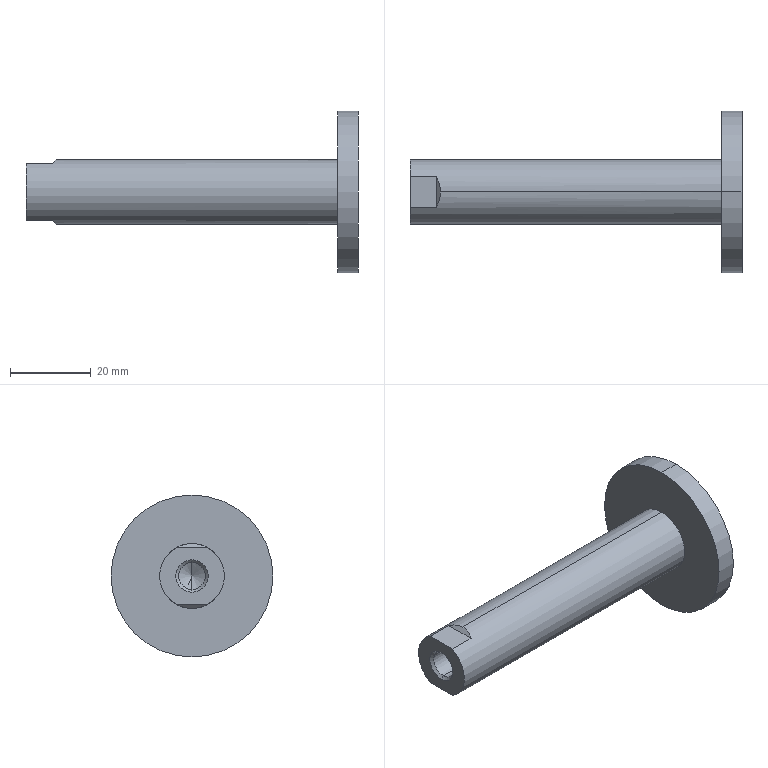Part | STEP file | _CDQ2F40-50-D-A93(0_0)_CYROD.stp | 1 solid | 17 faces | box 82 x 40 x 40 mm | volume 21214 mm3 | plane 7 | cylinder 6 | cone 4 | commonest cylinder face diameters 6.647 x2 16 x2 40 x2
STEP:
#1=CARTESIAN_POINT('',(0.,0.,0.));
#2=DIRECTION('',(0.,0.,1.));
#3=DIRECTION('',(1.,0.,0.));
#4=AXIS2_PLACEMENT_3D('',#1,#2,#3);
#5=CARTESIAN_POINT('',(-4.,0.,3.323));
#6=VERTEX_POINT('',#5);
#7=CARTESIAN_POINT('',(-4.,0.,-3.324));
#8=VERTEX_POINT('',#7);
#9=CARTESIAN_POINT('',(-4.,0.,0.));
#10=DIRECTION('',(1.,0.,0.));
#11=DIRECTION('',(0.,0.,-1.));
#12=AXIS2_PLACEMENT_3D('',#9,#10,#11);
#13=CIRCLE('',#12,3.324);
#14=CARTESIAN_POINT('',(-3.081,0.,0.));
#15=DIRECTION('',(-1.,0.,0.));
#16=DIRECTION('',(0.,0.,1.));
#17=AXIS2_PLACEMENT_3D('',#14,#15,#16);
#18=CONICAL_SURFACE('',#17,1.732,1.047);
#19=CARTESIAN_POINT('',(9.425,0.9188));
#20=DIRECTION('',(-1.,0.));
#21=VECTOR('',#20,1.);
#22=LINE('',#19,#21);
#23=(GEOMETRIC_REPRESENTATION_CONTEXT(2)PARAMETRIC_REPRESENTATION_CONTEXT()REPRESENTATION_CONTEXT('',''));
#24=DEFINITIONAL_REPRESENTATION('',(#22),#23);
#25=PCURVE('',#18,#24);
#26=CARTESIAN_POINT('',(65.,0.,0.));
#27=DIRECTION('',(-1.,0.,0.));
#28=DIRECTION('',(0.,0.,-1.));
#29=AXIS2_PLACEMENT_3D('',#26,#27,#28);
#30=CYLINDRICAL_SURFACE('',#29,3.324);
#31=CARTESIAN_POINT('',(6.283,69.));
#32=DIRECTION('',(-1.,0.));
#33=VECTOR('',#32,1.);
#34=LINE('',#31,#33);
#35=(GEOMETRIC_REPRESENTATION_CONTEXT(2)PARAMETRIC_REPRESENTATION_CONTEXT()REPRESENTATION_CONTEXT('',''));
#36=DEFINITIONAL_REPRESENTATION('',(#34),#35);
#37=PCURVE('',#30,#36);
#38=SURFACE_CURVE('',#13,(#25,#37),.PCURVE_S1.);
#39=EDGE_CURVE('',#6,#8,#38,.T.);
#40=ORIENTED_EDGE('',*,*,#39,.T.);
#41=CARTESIAN_POINT('',(-2.081,0.,0.));
#42=VERTEX_POINT('',#41);
#43=CARTESIAN_POINT('',(-3.081,0.,-1.732));
#44=DIRECTION('',(-0.5,0.,-0.866));
#45=VECTOR('',#44,1.);
#46=LINE('',#43,#45);
#47=CARTESIAN_POINT('',(3.142,0.));
#48=DIRECTION('',(0.,1.));
#49=VECTOR('',#48,1.);
#50=LINE('',#47,#49);
#51=(GEOMETRIC_REPRESENTATION_CONTEXT(2)PARAMETRIC_REPRESENTATION_CONTEXT()REPRESENTATION_CONTEXT('',''));
#52=DEFINITIONAL_REPRESENTATION('',(#50),#51);
#53=PCURVE('',#18,#52);
#54=CARTESIAN_POINT('',(-3.081,0.,0.));
#55=DIRECTION('',(-1.,0.,0.));
#56=DIRECTION('',(0.,0.,1.));
#57=AXIS2_PLACEMENT_3D('',#54,#55,#56);
#58=CONICAL_SURFACE('',#57,1.732,1.047);
#59=CARTESIAN_POINT('',(3.142,0.));
#60=DIRECTION('',(0.,1.));
#61=VECTOR('',#60,1.);
#62=LINE('',#59,#61);
#63=(GEOMETRIC_REPRESENTATION_CONTEXT(2)PARAMETRIC_REPRESENTATION_CONTEXT()REPRESENTATION_CONTEXT('',''));
#64=DEFINITIONAL_REPRESENTATION('',(#62),#63);
#65=PCURVE('',#58,#64);
#66=SURFACE_CURVE('',#46,(#53,#65),.PCURVE_S1.);
#67=EDGE_CURVE('',#42,#8,#66,.T.);
#68=ORIENTED_EDGE('',*,*,#67,.F.);
#69=CARTESIAN_POINT('',(-3.081,0.,1.732));
#70=DIRECTION('',(-0.5,0.,0.866));
#71=VECTOR('',#70,1.);
#72=LINE('',#69,#71);
#73=CARTESIAN_POINT('',(6.283,0.));
#74=DIRECTION('',(0.,1.));
#75=VECTOR('',#74,1.);
#76=LINE('',#73,#75);
#77=(GEOMETRIC_REPRESENTATION_CONTEXT(2)PARAMETRIC_REPRESENTATION_CONTEXT()REPRESENTATION_CONTEXT('',''));
#78=DEFINITIONAL_REPRESENTATION('',(#76),#77);
#79=PCURVE('',#18,#78);
#80=CARTESIAN_POINT('',(0.,0.));
#81=DIRECTION('',(0.,1.));
#82=VECTOR('',#81,1.);
#83=LINE('',#80,#82);
#84=(GEOMETRIC_REPRESENTATION_CONTEXT(2)PARAMETRIC_REPRESENTATION_CONTEXT()REPRESENTATION_CONTEXT('',''));
#85=DEFINITIONAL_REPRESENTATION('',(#83),#84);
#86=PCURVE('',#58,#85);
#87=SURFACE_CURVE('',#72,(#79,#86),.PCURVE_S1.);
#88=EDGE_CURVE('',#42,#6,#87,.T.);
#89=ORIENTED_EDGE('',*,*,#88,.T.);
#90=EDGE_LOOP('',(#40,#68,#89));
#91=FACE_BOUND('',#90,.F.);
#92=ADVANCED_FACE('',(#91),#18,.F.);
#93=CARTESIAN_POINT('',(-10.5,3.873,-7.));
#94=VERTEX_POINT('',#93);
#95=CARTESIAN_POINT('',(-9.5,0.,-8.));
#96=VERTEX_POINT('',#95);
#97=CARTESIAN_POINT('',(-10.5,3.873,-7.));
#98=CARTESIAN_POINT('',(-9.841,2.681,-7.659));
#99=CARTESIAN_POINT('',(-9.5,1.362,-8.));
#100=CARTESIAN_POINT('',(-9.5,0.,-8.));
#101=(BOUNDED_CURVE()B_SPLINE_CURVE(3,(#97,#98,#99,#100),.UNSPECIFIED.,.F.,.F.)B_SPLINE_CURVE_WITH_KNOTS((4,4),(5.778,6.283),.PIECEWISE_BEZIER_KNOTS.)CURVE()GEOMETRIC_REPRESENTATION_ITEM()RATIONAL_B_SPLINE_CURVE((1.,0.9788,0.9788,1.))REPRESENTATION_ITEM(''));
#102=CARTESIAN_POINT('',(-9.463,-4.26,-8.037));
#103=DIRECTION('',(-0.7071,0.,-0.7071));
#104=DIRECTION('',(-0.7071,0.,0.7071));
#105=AXIS2_PLACEMENT_3D('',#102,#103,#104);
#106=PLANE('',#105);
#107=CARTESIAN_POINT('',(1.466,8.133));
#108=CARTESIAN_POINT('',(0.5336,6.941));
#109=CARTESIAN_POINT('',(0.05199,5.622));
#110=CARTESIAN_POINT('',(0.05199,4.26));
#111=(BOUNDED_CURVE()B_SPLINE_CURVE(3,(#107,#108,#109,#110),.UNSPECIFIED.,.F.,.F.)B_SPLINE_CURVE_WITH_KNOTS((4,4),(5.778,6.283),.PIECEWISE_BEZIER_KNOTS.)CURVE()GEOMETRIC_REPRESENTATION_ITEM()RATIONAL_B_SPLINE_CURVE((1.,0.9788,0.9788,1.))REPRESENTATION_ITEM(''));
#112=(GEOMETRIC_REPRESENTATION_CONTEXT(2)PARAMETRIC_REPRESENTATION_CONTEXT()REPRESENTATION_CONTEXT('',''));
#113=DEFINITIONAL_REPRESENTATION('',(#111),#112);
#114=PCURVE('',#106,#113);
#115=CARTESIAN_POINT('',(65.,0.,0.));
#116=DIRECTION('',(-1.,0.,0.));
#117=DIRECTION('',(0.,0.,-1.));
#118=AXIS2_PLACEMENT_3D('',#115,#116,#117);
#119=CYLINDRICAL_SURFACE('',#118,8.);
#120=CARTESIAN_POINT('',(5.778,75.5));
#121=CARTESIAN_POINT('',(5.785,75.471));
#122=CARTESIAN_POINT('',(5.801,75.413));
#123=CARTESIAN_POINT('',(5.823,75.33));
#124=CARTESIAN_POINT('',(5.846,75.251));
#125=CARTESIAN_POINT('',(5.869,75.175));
#126=CARTESIAN_POINT('',(5.892,75.103));
#127=CARTESIAN_POINT('',(5.915,75.035));
#128=CARTESIAN_POINT('',(5.938,74.971));
#129=CARTESIAN_POINT('',(5.961,74.91));
#130=CARTESIAN_POINT('',(5.984,74.854));
#131=CARTESIAN_POINT('',(6.007,74.802));
#132=CARTESIAN_POINT('',(6.031,74.753));
#133=CARTESIAN_POINT('',(6.054,74.709));
#134=CARTESIAN_POINT('',(6.077,74.669));
#135=CARTESIAN_POINT('',(6.1,74.634));
#136=CARTESIAN_POINT('',(6.123,74.602));
#137=CARTESIAN_POINT('',(6.146,74.575));
#138=CARTESIAN_POINT('',(6.169,74.552));
#139=CARTESIAN_POINT('',(6.192,74.533));
#140=CARTESIAN_POINT('',(6.215,74.518));
#141=CARTESIAN_POINT('',(6.238,74.508));
#142=CARTESIAN_POINT('',(6.26,74.501));
#143=CARTESIAN_POINT('',(6.276,74.5));
#144=CARTESIAN_POINT('',(6.283,74.5));
#145=B_SPLINE_CURVE_WITH_KNOTS('',3,(#120,#121,#122,#123,#124,#125,#126,#127,#128,#129,#130,#131,#132,#133,#134,#135,#136,#137,#138,#139,#140,#141,#142,#143,#144),.UNSPECIFIED.,.F.,.F.,(4,1,1,1,1,1,1,1,1,1,1,1,1,1,1,1,1,1,1,1,1,1,4),(5.778,5.801,5.824,5.847,5.87,5.893,5.916,5.939,5.962,5.985,6.008,6.031,6.053,6.076,6.099,6.122,6.145,6.168,6.191,6.214,6.237,6.26,6.283),.QUASI_UNIFORM_KNOTS.);
#146=(GEOMETRIC_REPRESENTATION_CONTEXT(2)PARAMETRIC_REPRESENTATION_CONTEXT()REPRESENTATION_CONTEXT('',''));
#147=DEFINITIONAL_REPRESENTATION('',(#145),#146);
#148=PCURVE('',#119,#147);
#149=SURFACE_CURVE('',#101,(#114,#148),.PCURVE_S1.);
#150=EDGE_CURVE('',#94,#96,#149,.T.);
#151=ORIENTED_EDGE('',*,*,#150,.T.);
#152=CARTESIAN_POINT('',(-10.5,-3.873,-7.));
#153=VERTEX_POINT('',#152);
#154=CARTESIAN_POINT('',(-9.5,0.,-8.));
#155=CARTESIAN_POINT('',(-9.5,-1.362,-8.));
#156=CARTESIAN_POINT('',(-9.841,-2.681,-7.659));
#157=CARTESIAN_POINT('',(-10.5,-3.873,-7.));
#158=(BOUNDED_CURVE()B_SPLINE_CURVE(3,(#154,#155,#156,#157),.UNSPECIFIED.,.F.,.F.)B_SPLINE_CURVE_WITH_KNOTS((4,4),(0.,0.5054),.PIECEWISE_BEZIER_KNOTS.)CURVE()GEOMETRIC_REPRESENTATION_ITEM()RATIONAL_B_SPLINE_CURVE((1.,0.9788,0.9788,1.))REPRESENTATION_ITEM(''));
#159=CARTESIAN_POINT('',(0.05199,4.26));
#160=CARTESIAN_POINT('',(0.05199,2.898));
#161=CARTESIAN_POINT('',(0.5336,1.579));
#162=CARTESIAN_POINT('',(1.466,0.3873));
#163=(BOUNDED_CURVE()B_SPLINE_CURVE(3,(#159,#160,#161,#162),.UNSPECIFIED.,.F.,.F.)B_SPLINE_CURVE_WITH_KNOTS((4,4),(0.,0.5054),.PIECEWISE_BEZIER_KNOTS.)CURVE()GEOMETRIC_REPRESENTATION_ITEM()RATIONAL_B_SPLINE_CURVE((1.,0.9788,0.9788,1.))REPRESENTATION_ITEM(''));
#164=(GEOMETRIC_REPRESENTATION_CONTEXT(2)PARAMETRIC_REPRESENTATION_CONTEXT()REPRESENTATION_CONTEXT('',''));
#165=DEFINITIONAL_REPRESENTATION('',(#163),#164);
#166=PCURVE('',#106,#165);
#167=CARTESIAN_POINT('',(65.,0.,0.));
#168=DIRECTION('',(-1.,0.,0.));
#169=DIRECTION('',(0.,0.,-1.));
#170=AXIS2_PLACEMENT_3D('',#167,#168,#169);
#171=CYLINDRICAL_SURFACE('',#170,8.);
#172=CARTESIAN_POINT('',(0.,74.5));
#173=CARTESIAN_POINT('',(0.007576,74.5));
#174=CARTESIAN_POINT('',(0.02275,74.501));
#175=CARTESIAN_POINT('',(0.04557,74.508));
#176=CARTESIAN_POINT('',(0.06844,74.518));
#177=CARTESIAN_POINT('',(0.09137,74.533));
#178=CARTESIAN_POINT('',(0.1143,74.552));
#179=CARTESIAN_POINT('',(0.1373,74.575));
#180=CARTESIAN_POINT('',(0.1604,74.602));
#181=CARTESIAN_POINT('',(0.1834,74.634));
#182=CARTESIAN_POINT('',(0.2065,74.669));
#183=CARTESIAN_POINT('',(0.2296,74.709));
#184=CARTESIAN_POINT('',(0.2527,74.753));
#185=CARTESIAN_POINT('',(0.2758,74.802));
#186=CARTESIAN_POINT('',(0.2989,74.854));
#187=CARTESIAN_POINT('',(0.3219,74.91));
#188=CARTESIAN_POINT('',(0.345,74.971));
#189=CARTESIAN_POINT('',(0.368,75.035));
#190=CARTESIAN_POINT('',(0.391,75.103));
#191=CARTESIAN_POINT('',(0.414,75.175));
#192=CARTESIAN_POINT('',(0.4369,75.251));
#193=CARTESIAN_POINT('',(0.4598,75.33));
#194=CARTESIAN_POINT('',(0.4826,75.413));
#195=CARTESIAN_POINT('',(0.4978,75.471));
#196=CARTESIAN_POINT('',(0.5054,75.5));
#197=B_SPLINE_CURVE_WITH_KNOTS('',3,(#172,#173,#174,#175,#176,#177,#178,#179,#180,#181,#182,#183,#184,#185,#186,#187,#188,#189,#190,#191,#192,#193,#194,#195,#196),.UNSPECIFIED.,.F.,.F.,(4,1,1,1,1,1,1,1,1,1,1,1,1,1,1,1,1,1,1,1,1,1,4),(0.,0.02297,0.04594,0.06891,0.09188,0.1149,0.1378,0.1608,0.1838,0.2067,0.2297,0.2527,0.2757,0.2986,0.3216,0.3446,0.3675,0.3905,0.4135,0.4364,0.4594,0.4824,0.5054),.QUASI_UNIFORM_KNOTS.);
#198=(GEOMETRIC_REPRESENTATION_CONTEXT(2)PARAMETRIC_REPRESENTATION_CONTEXT()REPRESENTATION_CONTEXT('',''));
#199=DEFINITIONAL_REPRESENTATION('',(#197),#198);
#200=PCURVE('',#171,#199);
#201=SURFACE_CURVE('',#158,(#166,#200),.PCURVE_S1.);
#202=EDGE_CURVE('',#96,#153,#201,.T.);
#203=ORIENTED_EDGE('',*,*,#202,.T.);
#204=CARTESIAN_POINT('',(-10.5,3.873,-7.));
#205=DIRECTION('',(0.,-1.,0.));
#206=VECTOR('',#205,1.);
#207=LINE('',#204,#206);
#208=CARTESIAN_POINT('',(1.466,8.133));
#209=DIRECTION('',(0.,-1.));
#210=VECTOR('',#209,1.);
#211=LINE('',#208,#210);
#212=(GEOMETRIC_REPRESENTATION_CONTEXT(2)PARAMETRIC_REPRESENTATION_CONTEXT()REPRESENTATION_CONTEXT('',''));
#213=DEFINITIONAL_REPRESENTATION('',(#211),#212);
#214=PCURVE('',#106,#213);
#215=CARTESIAN_POINT('',(-10.175,-4.26,-7.));
#216=DIRECTION('',(0.,0.,-1.));
#217=DIRECTION('',(0.,-1.,0.));
#218=AXIS2_PLACEMENT_3D('',#215,#216,#217);
#219=PLANE('',#218);
#220=CARTESIAN_POINT('',(-8.133,0.325));
#221=DIRECTION('',(1.,0.));
#222=VECTOR('',#221,1.);
#223=LINE('',#220,#222);
#224=(GEOMETRIC_REPRESENTATION_CONTEXT(2)PARAMETRIC_REPRESENTATION_CONTEXT()REPRESENTATION_CONTEXT('',''));
#225=DEFINITIONAL_REPRESENTATION('',(#223),#224);
#226=PCURVE('',#219,#225);
#227=SURFACE_CURVE('',#207,(#214,#226),.PCURVE_S1.);
#228=EDGE_CURVE('',#94,#153,#227,.T.);
#229=ORIENTED_EDGE('',*,*,#228,.F.);
#230=EDGE_LOOP('',(#151,#203,#229));
#231=FACE_BOUND('',#230,.T.);
#232=ADVANCED_FACE('',(#231),#106,.T.);
#233=CARTESIAN_POINT('',(-17.,3.873,-7.));
#234=VERTEX_POINT('',#233);
#235=CARTESIAN_POINT('',(-17.,3.873,-7.));
#236=DIRECTION('',(1.,0.,0.));
#237=VECTOR('',#236,1.);
#238=LINE('',#235,#237);
#239=CARTESIAN_POINT('',(-8.133,6.825));
#240=DIRECTION('',(0.,-1.));
#241=VECTOR('',#240,1.);
#242=LINE('',#239,#241);
#243=(GEOMETRIC_REPRESENTATION_CONTEXT(2)PARAMETRIC_REPRESENTATION_CONTEXT()REPRESENTATION_CONTEXT('',''));
#244=DEFINITIONAL_REPRESENTATION('',(#242),#243);
#245=PCURVE('',#219,#244);
#246=CARTESIAN_POINT('',(5.778,82.));
#247=DIRECTION('',(0.,-1.));
#248=VECTOR('',#247,1.);
#249=LINE('',#246,#248);
#250=(GEOMETRIC_REPRESENTATION_CONTEXT(2)PARAMETRIC_REPRESENTATION_CONTEXT()REPRESENTATION_CONTEXT('',''));
#251=DEFINITIONAL_REPRESENTATION('',(#249),#250);
#252=PCURVE('',#119,#251);
#253=SURFACE_CURVE('',#238,(#245,#252),.PCURVE_S1.);
#254=EDGE_CURVE('',#234,#94,#253,.T.);
#255=ORIENTED_EDGE('',*,*,#254,.T.);
#256=ORIENTED_EDGE('',*,*,#228,.T.);
#257=CARTESIAN_POINT('',(-17.,-3.873,-7.));
#258=VERTEX_POINT('',#257);
#259=CARTESIAN_POINT('',(-17.,-3.873,-7.));
#260=DIRECTION('',(-1.,0.,0.));
#261=VECTOR('',#260,1.);
#262=LINE('',#259,#261);
#263=CARTESIAN_POINT('',(-0.3873,6.825));
#264=DIRECTION('',(0.,1.));
#265=VECTOR('',#264,1.);
#266=LINE('',#263,#265);
#267=(GEOMETRIC_REPRESENTATION_CONTEXT(2)PARAMETRIC_REPRESENTATION_CONTEXT()REPRESENTATION_CONTEXT('',''));
#268=DEFINITIONAL_REPRESENTATION('',(#266),#267);
#269=PCURVE('',#219,#268);
#270=CARTESIAN_POINT('',(0.5054,82.));
#271=DIRECTION('',(0.,1.));
#272=VECTOR('',#271,1.);
#273=LINE('',#270,#272);
#274=(GEOMETRIC_REPRESENTATION_CONTEXT(2)PARAMETRIC_REPRESENTATION_CONTEXT()REPRESENTATION_CONTEXT('',''));
#275=DEFINITIONAL_REPRESENTATION('',(#273),#274);
#276=PCURVE('',#171,#275);
#277=SURFACE_CURVE('',#262,(#269,#276),.PCURVE_S1.);
#278=EDGE_CURVE('',#153,#258,#277,.T.);
#279=ORIENTED_EDGE('',*,*,#278,.T.);
#280=CARTESIAN_POINT('',(-17.,3.873,-7.));
#281=DIRECTION('',(0.,-1.,0.));
#282=VECTOR('',#281,1.);
#283=LINE('',#280,#282);
#284=CARTESIAN_POINT('',(-8.133,6.825));
#285=DIRECTION('',(1.,0.));
#286=VECTOR('',#285,1.);
#287=LINE('',#284,#286);
#288=(GEOMETRIC_REPRESENTATION_CONTEXT(2)PARAMETRIC_REPRESENTATION_CONTEXT()REPRESENTATION_CONTEXT('',''));
#289=DEFINITIONAL_REPRESENTATION('',(#287),#288);
#290=PCURVE('',#219,#289);
#291=CARTESIAN_POINT('',(-17.,-8.8,7.7));
#292=DIRECTION('',(1.,0.,0.));
#293=DIRECTION('',(0.,1.,0.));
#294=AXIS2_PLACEMENT_3D('',#291,#292,#293);
#295=PLANE('',#294);
#296=CARTESIAN_POINT('',(12.673,-14.7));
#297=DIRECTION('',(-1.,0.));
#298=VECTOR('',#297,1.);
#299=LINE('',#296,#298);
#300=(GEOMETRIC_REPRESENTATION_CONTEXT(2)PARAMETRIC_REPRESENTATION_CONTEXT()REPRESENTATION_CONTEXT('',''));
#301=DEFINITIONAL_REPRESENTATION('',(#299),#300);
#302=PCURVE('',#295,#301);
#303=SURFACE_CURVE('',#283,(#290,#302),.PCURVE_S1.);
#304=EDGE_CURVE('',#234,#258,#303,.T.);
#305=ORIENTED_EDGE('',*,*,#304,.F.);
#306=EDGE_LOOP('',(#255,#256,#279,#305));
#307=FACE_BOUND('',#306,.T.);
#308=ADVANCED_FACE('',(#307),#219,.T.);
#309=CARTESIAN_POINT('',(-17.,-3.873,7.));
#310=VERTEX_POINT('',#309);
#311=CARTESIAN_POINT('',(-10.5,-3.873,7.));
#312=VERTEX_POINT('',#311);
#313=CARTESIAN_POINT('',(-17.,-3.873,7.));
#314=DIRECTION('',(1.,0.,0.));
#315=VECTOR('',#314,1.);
#316=LINE('',#313,#315);
#317=CARTESIAN_POINT('',(-17.325,-4.26,7.));
#318=DIRECTION('',(0.,0.,1.));
#319=DIRECTION('',(1.,0.,0.));
#320=AXIS2_PLACEMENT_3D('',#317,#318,#319);
#321=PLANE('',#320);
#322=CARTESIAN_POINT('',(0.325,0.3873));
#323=DIRECTION('',(1.,0.));
#324=VECTOR('',#323,1.);
#325=LINE('',#322,#324);
#326=(GEOMETRIC_REPRESENTATION_CONTEXT(2)PARAMETRIC_REPRESENTATION_CONTEXT()REPRESENTATION_CONTEXT('',''));
#327=DEFINITIONAL_REPRESENTATION('',(#325),#326);
#328=PCURVE('',#321,#327);
#329=CARTESIAN_POINT('',(2.636,82.));
#330=DIRECTION('',(0.,-1.));
#331=VECTOR('',#330,1.);
#332=LINE('',#329,#331);
#333=(GEOMETRIC_REPRESENTATION_CONTEXT(2)PARAMETRIC_REPRESENTATION_CONTEXT()REPRESENTATION_CONTEXT('',''));
#334=DEFINITIONAL_REPRESENTATION('',(#332),#333);
#335=PCURVE('',#171,#334);
#336=SURFACE_CURVE('',#316,(#328,#335),.PCURVE_S1.);
#337=EDGE_CURVE('',#310,#312,#336,.T.);
#338=ORIENTED_EDGE('',*,*,#337,.T.);
#339=CARTESIAN_POINT('',(-10.5,3.873,7.));
#340=VERTEX_POINT('',#339);
#341=CARTESIAN_POINT('',(-10.5,3.873,7.));
#342=DIRECTION('',(0.,-1.,0.));
#343=VECTOR('',#342,1.);
#344=LINE('',#341,#343);
#345=CARTESIAN_POINT('',(6.825,8.133));
#346=DIRECTION('',(0.,-1.));
#347=VECTOR('',#346,1.);
#348=LINE('',#345,#347);
#349=(GEOMETRIC_REPRESENTATION_CONTEXT(2)PARAMETRIC_REPRESENTATION_CONTEXT()REPRESENTATION_CONTEXT('',''));
#350=DEFINITIONAL_REPRESENTATION('',(#348),#349);
#351=PCURVE('',#321,#350);
#352=CARTESIAN_POINT('',(-10.549,-4.26,6.951));
#353=DIRECTION('',(-0.7071,0.,0.7071));
#354=DIRECTION('',(0.,1.,0.));
#355=AXIS2_PLACEMENT_3D('',#352,#353,#354);
#356=PLANE('',#355);
#357=CARTESIAN_POINT('',(8.133,-0.06982));
#358=DIRECTION('',(-1.,0.));
#359=VECTOR('',#358,1.);
#360=LINE('',#357,#359);
#361=(GEOMETRIC_REPRESENTATION_CONTEXT(2)PARAMETRIC_REPRESENTATION_CONTEXT()REPRESENTATION_CONTEXT('',''));
#362=DEFINITIONAL_REPRESENTATION('',(#360),#361);
#363=PCURVE('',#356,#362);
#364=SURFACE_CURVE('',#344,(#351,#363),.PCURVE_S1.);
#365=EDGE_CURVE('',#340,#312,#364,.T.);
#366=ORIENTED_EDGE('',*,*,#365,.F.);
#367=CARTESIAN_POINT('',(-17.,3.873,7.));
#368=VERTEX_POINT('',#367);
#369=CARTESIAN_POINT('',(-17.,3.873,7.));
#370=DIRECTION('',(-1.,0.,0.));
#371=VECTOR('',#370,1.);
#372=LINE('',#369,#371);
#373=CARTESIAN_POINT('',(0.325,8.133));
#374=DIRECTION('',(-1.,0.));
#375=VECTOR('',#374,1.);
#376=LINE('',#373,#375);
#377=(GEOMETRIC_REPRESENTATION_CONTEXT(2)PARAMETRIC_REPRESENTATION_CONTEXT()REPRESENTATION_CONTEXT('',''));
#378=DEFINITIONAL_REPRESENTATION('',(#376),#377);
#379=PCURVE('',#321,#378);
#380=CARTESIAN_POINT('',(3.647,82.));
#381=DIRECTION('',(0.,1.));
#382=VECTOR('',#381,1.);
#383=LINE('',#380,#382);
#384=(GEOMETRIC_REPRESENTATION_CONTEXT(2)PARAMETRIC_REPRESENTATION_CONTEXT()REPRESENTATION_CONTEXT('',''));
#385=DEFINITIONAL_REPRESENTATION('',(#383),#384);
#386=PCURVE('',#119,#385);
#387=SURFACE_CURVE('',#372,(#379,#386),.PCURVE_S1.);
#388=EDGE_CURVE('',#340,#368,#387,.T.);
#389=ORIENTED_EDGE('',*,*,#388,.T.);
#390=CARTESIAN_POINT('',(-17.,3.873,7.));
#391=DIRECTION('',(0.,-1.,0.));
#392=VECTOR('',#391,1.);
#393=LINE('',#390,#392);
#394=CARTESIAN_POINT('',(0.325,8.133));
#395=DIRECTION('',(0.,-1.));
#396=VECTOR('',#395,1.);
#397=LINE('',#394,#396);
#398=(GEOMETRIC_REPRESENTATION_CONTEXT(2)PARAMETRIC_REPRESENTATION_CONTEXT()REPRESENTATION_CONTEXT('',''));
#399=DEFINITIONAL_REPRESENTATION('',(#397),#398);
#400=PCURVE('',#321,#399);
#401=CARTESIAN_POINT('',(12.673,-0.7));
#402=DIRECTION('',(-1.,0.));
#403=VECTOR('',#402,1.);
#404=LINE('',#401,#403);
#405=(GEOMETRIC_REPRESENTATION_CONTEXT(2)PARAMETRIC_REPRESENTATION_CONTEXT()REPRESENTATION_CONTEXT('',''));
#406=DEFINITIONAL_REPRESENTATION('',(#404),#405);
#407=PCURVE('',#295,#406);
#408=SURFACE_CURVE('',#393,(#400,#407),.PCURVE_S1.);
#409=EDGE_CURVE('',#368,#310,#408,.T.);
#410=ORIENTED_EDGE('',*,*,#409,.T.);
#411=EDGE_LOOP('',(#338,#366,#389,#410));
#412=FACE_BOUND('',#411,.T.);
#413=ADVANCED_FACE('',(#412),#321,.T.);
#414=CARTESIAN_POINT('',(-9.5,0.,8.));
#415=VERTEX_POINT('',#414);
#416=CARTESIAN_POINT('',(-10.5,-3.873,7.));
#417=CARTESIAN_POINT('',(-9.841,-2.681,7.659));
#418=CARTESIAN_POINT('',(-9.5,-1.362,8.));
#419=CARTESIAN_POINT('',(-9.5,0.,8.));
#420=(BOUNDED_CURVE()B_SPLINE_CURVE(3,(#416,#417,#418,#419),.UNSPECIFIED.,.F.,.F.)B_SPLINE_CURVE_WITH_KNOTS((4,4),(5.778,6.283),.PIECEWISE_BEZIER_KNOTS.)CURVE()GEOMETRIC_REPRESENTATION_ITEM()RATIONAL_B_SPLINE_CURVE((1.,0.9788,0.9788,1.))REPRESENTATION_ITEM(''));
#421=CARTESIAN_POINT('',(0.3873,-0.06982));
#422=CARTESIAN_POINT('',(1.579,-1.002));
#423=CARTESIAN_POINT('',(2.898,-1.484));
#424=CARTESIAN_POINT('',(4.26,-1.484));
#425=(BOUNDED_CURVE()B_SPLINE_CURVE(3,(#421,#422,#423,#424),.UNSPECIFIED.,.F.,.F.)B_SPLINE_CURVE_WITH_KNOTS((4,4),(5.778,6.283),.PIECEWISE_BEZIER_KNOTS.)CURVE()GEOMETRIC_REPRESENTATION_ITEM()RATIONAL_B_SPLINE_CURVE((1.,0.9788,0.9788,1.))REPRESENTATION_ITEM(''));
#426=(GEOMETRIC_REPRESENTATION_CONTEXT(2)PARAMETRIC_REPRESENTATION_CONTEXT()REPRESENTATION_CONTEXT('',''));
#427=DEFINITIONAL_REPRESENTATION('',(#425),#426);
#428=PCURVE('',#356,#427);
#429=CARTESIAN_POINT('',(2.636,75.5));
#430=CARTESIAN_POINT('',(2.644,75.471));
#431=CARTESIAN_POINT('',(2.659,75.413));
#432=CARTESIAN_POINT('',(2.682,75.33));
#433=CARTESIAN_POINT('',(2.705,75.251));
#434=CARTESIAN_POINT('',(2.728,75.175));
#435=CARTESIAN_POINT('',(2.751,75.103));
#436=CARTESIAN_POINT('',(2.774,75.035));
#437=CARTESIAN_POINT('',(2.797,74.971));
#438=CARTESIAN_POINT('',(2.82,74.91));
#439=CARTESIAN_POINT('',(2.843,74.854));
#440=CARTESIAN_POINT('',(2.866,74.802));
#441=CARTESIAN_POINT('',(2.889,74.753));
#442=CARTESIAN_POINT('',(2.912,74.709));
#443=CARTESIAN_POINT('',(2.935,74.669));
#444=CARTESIAN_POINT('',(2.958,74.634));
#445=CARTESIAN_POINT('',(2.981,74.602));
#446=CARTESIAN_POINT('',(3.004,74.575));
#447=CARTESIAN_POINT('',(3.027,74.552));
#448=CARTESIAN_POINT('',(3.05,74.533));
#449=CARTESIAN_POINT('',(3.073,74.518));
#450=CARTESIAN_POINT('',(3.096,74.508));
#451=CARTESIAN_POINT('',(3.119,74.501));
#452=CARTESIAN_POINT('',(3.134,74.5));
#453=CARTESIAN_POINT('',(3.142,74.5));
#454=B_SPLINE_CURVE_WITH_KNOTS('',3,(#429,#430,#431,#432,#433,#434,#435,#436,#437,#438,#439,#440,#441,#442,#443,#444,#445,#446,#447,#448,#449,#450,#451,#452,#453),.UNSPECIFIED.,.F.,.F.,(4,1,1,1,1,1,1,1,1,1,1,1,1,1,1,1,1,1,1,1,1,1,4),(5.778,5.801,5.824,5.847,5.87,5.893,5.916,5.939,5.962,5.985,6.008,6.031,6.053,6.076,6.099,6.122,6.145,6.168,6.191,6.214,6.237,6.26,6.283),.QUASI_UNIFORM_KNOTS.);
#455=(GEOMETRIC_REPRESENTATION_CONTEXT(2)PARAMETRIC_REPRESENTATION_CONTEXT()REPRESENTATION_CONTEXT('',''));
#456=DEFINITIONAL_REPRESENTATION('',(#454),#455);
#457=PCURVE('',#171,#456);
#458=SURFACE_CURVE('',#420,(#428,#457),.PCURVE_S1.);
#459=EDGE_CURVE('',#312,#415,#458,.T.);
#460=ORIENTED_EDGE('',*,*,#459,.T.);
#461=CARTESIAN_POINT('',(-9.5,0.,8.));
#462=CARTESIAN_POINT('',(-9.5,1.362,8.));
#463=CARTESIAN_POINT('',(-9.841,2.681,7.659));
#464=CARTESIAN_POINT('',(-10.5,3.873,7.));
#465=(BOUNDED_CURVE()B_SPLINE_CURVE(3,(#461,#462,#463,#464),.UNSPECIFIED.,.F.,.F.)B_SPLINE_CURVE_WITH_KNOTS((4,4),(0.,0.5054),.PIECEWISE_BEZIER_KNOTS.)CURVE()GEOMETRIC_REPRESENTATION_ITEM()RATIONAL_B_SPLINE_CURVE((1.,0.9788,0.9788,1.))REPRESENTATION_ITEM(''));
#466=CARTESIAN_POINT('',(4.26,-1.484));
#467=CARTESIAN_POINT('',(5.622,-1.484));
#468=CARTESIAN_POINT('',(6.941,-1.002));
#469=CARTESIAN_POINT('',(8.133,-0.06982));
#470=(BOUNDED_CURVE()B_SPLINE_CURVE(3,(#466,#467,#468,#469),.UNSPECIFIED.,.F.,.F.)B_SPLINE_CURVE_WITH_KNOTS((4,4),(0.,0.5054),.PIECEWISE_BEZIER_KNOTS.)CURVE()GEOMETRIC_REPRESENTATION_ITEM()RATIONAL_B_SPLINE_CURVE((1.,0.9788,0.9788,1.))REPRESENTATION_ITEM(''));
#471=(GEOMETRIC_REPRESENTATION_CONTEXT(2)PARAMETRIC_REPRESENTATION_CONTEXT()REPRESENTATION_CONTEXT('',''));
#472=DEFINITIONAL_REPRESENTATION('',(#470),#471);
#473=PCURVE('',#356,#472);
#474=CARTESIAN_POINT('',(3.142,74.5));
#475=CARTESIAN_POINT('',(3.149,74.5));
#476=CARTESIAN_POINT('',(3.164,74.501));
#477=CARTESIAN_POINT('',(3.187,74.508));
#478=CARTESIAN_POINT('',(3.21,74.518));
#479=CARTESIAN_POINT('',(3.233,74.533));
#480=CARTESIAN_POINT('',(3.256,74.552));
#481=CARTESIAN_POINT('',(3.279,74.575));
#482=CARTESIAN_POINT('',(3.302,74.602));
#483=CARTESIAN_POINT('',(3.325,74.634));
#484=CARTESIAN_POINT('',(3.348,74.669));
#485=CARTESIAN_POINT('',(3.371,74.709));
#486=CARTESIAN_POINT('',(3.394,74.753));
#487=CARTESIAN_POINT('',(3.417,74.802));
#488=CARTESIAN_POINT('',(3.44,74.854));
#489=CARTESIAN_POINT('',(3.464,74.91));
#490=CARTESIAN_POINT('',(3.487,74.971));
#491=CARTESIAN_POINT('',(3.51,75.035));
#492=CARTESIAN_POINT('',(3.533,75.103));
#493=CARTESIAN_POINT('',(3.556,75.175));
#494=CARTESIAN_POINT('',(3.579,75.251));
#495=CARTESIAN_POINT('',(3.601,75.33));
#496=CARTESIAN_POINT('',(3.624,75.413));
#497=CARTESIAN_POINT('',(3.639,75.471));
#498=CARTESIAN_POINT('',(3.647,75.5));
#499=B_SPLINE_CURVE_WITH_KNOTS('',3,(#474,#475,#476,#477,#478,#479,#480,#481,#482,#483,#484,#485,#486,#487,#488,#489,#490,#491,#492,#493,#494,#495,#496,#497,#498),.UNSPECIFIED.,.F.,.F.,(4,1,1,1,1,1,1,1,1,1,1,1,1,1,1,1,1,1,1,1,1,1,4),(0.,0.02297,0.04594,0.06891,0.09188,0.1149,0.1378,0.1608,0.1838,0.2067,0.2297,0.2527,0.2757,0.2986,0.3216,0.3446,0.3675,0.3905,0.4135,0.4364,0.4594,0.4824,0.5054),.QUASI_UNIFORM_KNOTS.);
#500=(GEOMETRIC_REPRESENTATION_CONTEXT(2)PARAMETRIC_REPRESENTATION_CONTEXT()REPRESENTATION_CONTEXT('',''));
#501=DEFINITIONAL_REPRESENTATION('',(#499),#500);
#502=PCURVE('',#119,#501);
#503=SURFACE_CURVE('',#465,(#473,#502),.PCURVE_S1.);
#504=EDGE_CURVE('',#415,#340,#503,.T.);
#505=ORIENTED_EDGE('',*,*,#504,.T.);
#506=ORIENTED_EDGE('',*,*,#365,.T.);
#507=EDGE_LOOP('',(#460,#505,#506));
#508=FACE_BOUND('',#507,.T.);
#509=ADVANCED_FACE('',(#508),#356,.T.);
#510=CARTESIAN_POINT('',(65.,0.,-20.));
#511=VERTEX_POINT('',#510);
#512=CARTESIAN_POINT('',(65.,0.,20.));
#513=VERTEX_POINT('',#512);
#514=CARTESIAN_POINT('',(65.,0.,0.));
#515=DIRECTION('',(1.,0.,0.));
#516=DIRECTION('',(0.,0.,-1.));
#517=AXIS2_PLACEMENT_3D('',#514,#515,#516);
#518=CIRCLE('',#517,20.);
#519=CARTESIAN_POINT('',(65.,-22.,-22.));
#520=DIRECTION('',(-1.,0.,0.));
#521=DIRECTION('',(0.,0.,1.));
#522=AXIS2_PLACEMENT_3D('',#519,#520,#521);
#523=PLANE('',#522);
#524=CARTESIAN_POINT('',(2.,22.));
#525=CARTESIAN_POINT('',(2.,56.641));
#526=CARTESIAN_POINT('',(32.,39.321));
#527=CARTESIAN_POINT('',(62.,22.));
#528=CARTESIAN_POINT('',(32.,4.679));
#529=CARTESIAN_POINT('',(2.,-12.641));
#530=CARTESIAN_POINT('',(2.,22.));
#531=(BOUNDED_CURVE()B_SPLINE_CURVE(2,(#524,#525,#526,#527,#528,#529,#530),.UNSPECIFIED.,.T.,.F.)B_SPLINE_CURVE_WITH_KNOTS((1,2,2,2,2,1),(-2.094,0.,2.094,4.189,6.283,8.378),.UNSPECIFIED.)CURVE()GEOMETRIC_REPRESENTATION_ITEM()RATIONAL_B_SPLINE_CURVE((1.,0.5,1.,0.5,1.,0.5,1.))REPRESENTATION_ITEM(''));
#532=(GEOMETRIC_REPRESENTATION_CONTEXT(2)PARAMETRIC_REPRESENTATION_CONTEXT()REPRESENTATION_CONTEXT('',''));
#533=DEFINITIONAL_REPRESENTATION('',(#531),#532);
#534=PCURVE('',#523,#533);
#535=CARTESIAN_POINT('',(65.25,0.,0.));
#536=DIRECTION('',(-1.,0.,0.));
#537=DIRECTION('',(0.,0.,-1.));
#538=AXIS2_PLACEMENT_3D('',#535,#536,#537);
#539=CYLINDRICAL_SURFACE('',#538,20.);
#540=CARTESIAN_POINT('',(6.283,0.25));
#541=DIRECTION('',(-1.,0.));
#542=VECTOR('',#541,1.);
#543=LINE('',#540,#542);
#544=(GEOMETRIC_REPRESENTATION_CONTEXT(2)PARAMETRIC_REPRESENTATION_CONTEXT()REPRESENTATION_CONTEXT('',''));
#545=DEFINITIONAL_REPRESENTATION('',(#543),#544);
#546=PCURVE('',#539,#545);
#547=SURFACE_CURVE('',#518,(#534,#546),.PCURVE_S1.);
#548=EDGE_CURVE('',#511,#513,#547,.T.);
#549=ORIENTED_EDGE('',*,*,#548,.T.);
#550=CARTESIAN_POINT('',(65.,0.,0.));
#551=DIRECTION('',(1.,0.,0.));
#552=DIRECTION('',(0.,0.,-1.));
#553=AXIS2_PLACEMENT_3D('',#550,#551,#552);
#554=CIRCLE('',#553,20.);
#555=CARTESIAN_POINT('',(2.,22.));
#556=CARTESIAN_POINT('',(2.,56.641));
#557=CARTESIAN_POINT('',(32.,39.321));
#558=CARTESIAN_POINT('',(62.,22.));
#559=CARTESIAN_POINT('',(32.,4.679));
#560=CARTESIAN_POINT('',(2.,-12.641));
#561=CARTESIAN_POINT('',(2.,22.));
#562=(BOUNDED_CURVE()B_SPLINE_CURVE(2,(#555,#556,#557,#558,#559,#560,#561),.UNSPECIFIED.,.T.,.F.)B_SPLINE_CURVE_WITH_KNOTS((1,2,2,2,2,1),(-2.094,0.,2.094,4.189,6.283,8.378),.UNSPECIFIED.)CURVE()GEOMETRIC_REPRESENTATION_ITEM()RATIONAL_B_SPLINE_CURVE((1.,0.5,1.,0.5,1.,0.5,1.))REPRESENTATION_ITEM(''));
#563=(GEOMETRIC_REPRESENTATION_CONTEXT(2)PARAMETRIC_REPRESENTATION_CONTEXT()REPRESENTATION_CONTEXT('',''));
#564=DEFINITIONAL_REPRESENTATION('',(#562),#563);
#565=PCURVE('',#523,#564);
#566=CARTESIAN_POINT('',(65.25,0.,0.));
#567=DIRECTION('',(-1.,0.,0.));
#568=DIRECTION('',(0.,0.,-1.));
#569=AXIS2_PLACEMENT_3D('',#566,#567,#568);
#570=CYLINDRICAL_SURFACE('',#569,20.);
#571=CARTESIAN_POINT('',(6.283,0.25));
#572=DIRECTION('',(-1.,0.));
#573=VECTOR('',#572,1.);
#574=LINE('',#571,#573);
#575=(GEOMETRIC_REPRESENTATION_CONTEXT(2)PARAMETRIC_REPRESENTATION_CONTEXT()REPRESENTATION_CONTEXT('',''));
#576=DEFINITIONAL_REPRESENTATION('',(#574),#575);
#577=PCURVE('',#570,#576);
#578=SURFACE_CURVE('',#554,(#565,#577),.PCURVE_S1.);
#579=EDGE_CURVE('',#513,#511,#578,.T.);
#580=ORIENTED_EDGE('',*,*,#579,.T.);
#581=EDGE_LOOP('',(#549,#580));
#582=FACE_BOUND('',#581,.T.);
#583=ADVANCED_FACE('',(#582),#523,.F.);
#584=CARTESIAN_POINT('',(60.,0.,-20.));
#585=VERTEX_POINT('',#584);
#586=CARTESIAN_POINT('',(60.,0.,-20.));
#587=DIRECTION('',(1.,0.,0.));
#588=VECTOR('',#587,1.);
#589=LINE('',#586,#588);
#590=CARTESIAN_POINT('',(0.,5.25));
#591=DIRECTION('',(0.,-1.));
#592=VECTOR('',#591,1.);
#593=LINE('',#590,#592);
#594=(GEOMETRIC_REPRESENTATION_CONTEXT(2)PARAMETRIC_REPRESENTATION_CONTEXT()REPRESENTATION_CONTEXT('',''));
#595=DEFINITIONAL_REPRESENTATION('',(#593),#594);
#596=PCURVE('',#570,#595);
#597=CARTESIAN_POINT('',(6.283,5.25));
#598=DIRECTION('',(0.,-1.));
#599=VECTOR('',#598,1.);
#600=LINE('',#597,#599);
#601=(GEOMETRIC_REPRESENTATION_CONTEXT(2)PARAMETRIC_REPRESENTATION_CONTEXT()REPRESENTATION_CONTEXT('',''));
#602=DEFINITIONAL_REPRESENTATION('',(#600),#601);
#603=PCURVE('',#539,#602);
#604=SURFACE_CURVE('',#589,(#596,#603),.PCURVE_S1.);
#605=EDGE_CURVE('',#585,#511,#604,.T.);
#606=ORIENTED_EDGE('',*,*,#605,.T.);
#607=ORIENTED_EDGE('',*,*,#579,.F.);
#608=CARTESIAN_POINT('',(60.,0.,20.));
#609=VERTEX_POINT('',#608);
#610=CARTESIAN_POINT('',(60.,0.,20.));
#611=DIRECTION('',(1.,0.,0.));
#612=VECTOR('',#611,1.);
#613=LINE('',#610,#612);
#614=CARTESIAN_POINT('',(3.142,5.25));
#615=DIRECTION('',(0.,-1.));
#616=VECTOR('',#615,1.);
#617=LINE('',#614,#616);
#618=(GEOMETRIC_REPRESENTATION_CONTEXT(2)PARAMETRIC_REPRESENTATION_CONTEXT()REPRESENTATION_CONTEXT('',''));
#619=DEFINITIONAL_REPRESENTATION('',(#617),#618);
#620=PCURVE('',#570,#619);
#621=CARTESIAN_POINT('',(3.142,5.25));
#622=DIRECTION('',(0.,-1.));
#623=VECTOR('',#622,1.);
#624=LINE('',#621,#623);
#625=(GEOMETRIC_REPRESENTATION_CONTEXT(2)PARAMETRIC_REPRESENTATION_CONTEXT()REPRESENTATION_CONTEXT('',''));
#626=DEFINITIONAL_REPRESENTATION('',(#624),#625);
#627=PCURVE('',#539,#626);
#628=SURFACE_CURVE('',#613,(#620,#627),.PCURVE_S1.);
#629=EDGE_CURVE('',#609,#513,#628,.T.);
#630=ORIENTED_EDGE('',*,*,#629,.F.);
#631=CARTESIAN_POINT('',(60.,0.,0.));
#632=DIRECTION('',(1.,0.,0.));
#633=DIRECTION('',(0.,0.,-1.));
#634=AXIS2_PLACEMENT_3D('',#631,#632,#633);
#635=CIRCLE('',#634,20.);
#636=CARTESIAN_POINT('',(6.283,5.25));
#637=DIRECTION('',(-1.,0.));
#638=VECTOR('',#637,1.);
#639=LINE('',#636,#638);
#640=(GEOMETRIC_REPRESENTATION_CONTEXT(2)PARAMETRIC_REPRESENTATION_CONTEXT()REPRESENTATION_CONTEXT('',''));
#641=DEFINITIONAL_REPRESENTATION('',(#639),#640);
#642=PCURVE('',#570,#641);
#643=CARTESIAN_POINT('',(60.,-22.,22.));
#644=DIRECTION('',(1.,0.,0.));
#645=DIRECTION('',(0.,1.,0.));
#646=AXIS2_PLACEMENT_3D('',#643,#644,#645);
#647=PLANE('',#646);
#648=CARTESIAN_POINT('',(22.,-22.));
#649=DIRECTION('',(0.,-1.));
#650=AXIS2_PLACEMENT_2D('',#648,#649);
#651=CIRCLE('',#650,20.);
#652=(GEOMETRIC_REPRESENTATION_CONTEXT(2)PARAMETRIC_REPRESENTATION_CONTEXT()REPRESENTATION_CONTEXT('',''));
#653=DEFINITIONAL_REPRESENTATION('',(#651),#652);
#654=PCURVE('',#647,#653);
#655=SURFACE_CURVE('',#635,(#642,#654),.PCURVE_S1.);
#656=EDGE_CURVE('',#609,#585,#655,.T.);
#657=ORIENTED_EDGE('',*,*,#656,.T.);
#658=EDGE_LOOP('',(#606,#607,#630,#657));
#659=FACE_BOUND('',#658,.T.);
#660=ADVANCED_FACE('',(#659),#570,.T.);
#661=CARTESIAN_POINT('',(60.,0.,-8.));
#662=VERTEX_POINT('',#661);
#663=CARTESIAN_POINT('',(60.,0.,8.));
#664=VERTEX_POINT('',#663);
#665=CARTESIAN_POINT('',(60.,0.,0.));
#666=DIRECTION('',(1.,0.,0.));
#667=DIRECTION('',(0.,0.,-1.));
#668=AXIS2_PLACEMENT_3D('',#665,#666,#667);
#669=CIRCLE('',#668,8.);
#670=CARTESIAN_POINT('',(22.,-22.));
#671=DIRECTION('',(0.,-1.));
#672=AXIS2_PLACEMENT_2D('',#670,#671);
#673=CIRCLE('',#672,8.);
#674=(GEOMETRIC_REPRESENTATION_CONTEXT(2)PARAMETRIC_REPRESENTATION_CONTEXT()REPRESENTATION_CONTEXT('',''));
#675=DEFINITIONAL_REPRESENTATION('',(#673),#674);
#676=PCURVE('',#647,#675);
#677=CARTESIAN_POINT('',(6.283,5.));
#678=DIRECTION('',(-1.,0.));
#679=VECTOR('',#678,1.);
#680=LINE('',#677,#679);
#681=(GEOMETRIC_REPRESENTATION_CONTEXT(2)PARAMETRIC_REPRESENTATION_CONTEXT()REPRESENTATION_CONTEXT('',''));
#682=DEFINITIONAL_REPRESENTATION('',(#680),#681);
#683=PCURVE('',#119,#682);
#684=SURFACE_CURVE('',#669,(#676,#683),.PCURVE_S1.);
#685=EDGE_CURVE('',#662,#664,#684,.T.);
#686=ORIENTED_EDGE('',*,*,#685,.T.);
#687=CARTESIAN_POINT('',(60.,0.,0.));
#688=DIRECTION('',(1.,0.,0.));
#689=DIRECTION('',(0.,0.,-1.));
#690=AXIS2_PLACEMENT_3D('',#687,#688,#689);
#691=CIRCLE('',#690,8.);
#692=CARTESIAN_POINT('',(22.,-22.));
#693=DIRECTION('',(0.,-1.));
#694=AXIS2_PLACEMENT_2D('',#692,#693);
#695=CIRCLE('',#694,8.);
#696=(GEOMETRIC_REPRESENTATION_CONTEXT(2)PARAMETRIC_REPRESENTATION_CONTEXT()REPRESENTATION_CONTEXT('',''));
#697=DEFINITIONAL_REPRESENTATION('',(#695),#696);
#698=PCURVE('',#647,#697);
#699=CARTESIAN_POINT('',(6.283,5.));
#700=DIRECTION('',(-1.,0.));
#701=VECTOR('',#700,1.);
#702=LINE('',#699,#701);
#703=(GEOMETRIC_REPRESENTATION_CONTEXT(2)PARAMETRIC_REPRESENTATION_CONTEXT()REPRESENTATION_CONTEXT('',''));
#704=DEFINITIONAL_REPRESENTATION('',(#702),#703);
#705=PCURVE('',#171,#704);
#706=SURFACE_CURVE('',#691,(#698,#705),.PCURVE_S1.);
#707=EDGE_CURVE('',#664,#662,#706,.T.);
#708=ORIENTED_EDGE('',*,*,#707,.T.);
#709=EDGE_LOOP('',(#686,#708));
#710=FACE_BOUND('',#709,.T.);
#711=CARTESIAN_POINT('',(60.,0.,0.));
#712=DIRECTION('',(1.,0.,0.));
#713=DIRECTION('',(0.,0.,-1.));
#714=AXIS2_PLACEMENT_3D('',#711,#712,#713);
#715=CIRCLE('',#714,20.);
#716=CARTESIAN_POINT('',(22.,-22.));
#717=DIRECTION('',(0.,-1.));
#718=AXIS2_PLACEMENT_2D('',#716,#717);
#719=CIRCLE('',#718,20.);
#720=(GEOMETRIC_REPRESENTATION_CONTEXT(2)PARAMETRIC_REPRESENTATION_CONTEXT()REPRESENTATION_CONTEXT('',''));
#721=DEFINITIONAL_REPRESENTATION('',(#719),#720);
#722=PCURVE('',#647,#721);
#723=CARTESIAN_POINT('',(6.283,5.25));
#724=DIRECTION('',(-1.,0.));
#725=VECTOR('',#724,1.);
#726=LINE('',#723,#725);
#727=(GEOMETRIC_REPRESENTATION_CONTEXT(2)PARAMETRIC_REPRESENTATION_CONTEXT()REPRESENTATION_CONTEXT('',''));
#728=DEFINITIONAL_REPRESENTATION('',(#726),#727);
#729=PCURVE('',#539,#728);
#730=SURFACE_CURVE('',#715,(#722,#729),.PCURVE_S1.);
#731=EDGE_CURVE('',#585,#609,#730,.T.);
#732=ORIENTED_EDGE('',*,*,#731,.F.);
#733=ORIENTED_EDGE('',*,*,#656,.F.);
#734=EDGE_LOOP('',(#732,#733));
#735=FACE_BOUND('',#734,.T.);
#736=ADVANCED_FACE('',(#710,#735),#647,.F.);
#737=CARTESIAN_POINT('',(-16.323,0.,-3.324));
#738=VERTEX_POINT('',#737);
#739=CARTESIAN_POINT('',(-16.323,0.,3.324));
#740=VERTEX_POINT('',#739);
#741=CARTESIAN_POINT('',(-16.323,0.,0.));
#742=DIRECTION('',(1.,0.,0.));
#743=DIRECTION('',(0.,0.,-1.));
#744=AXIS2_PLACEMENT_3D('',#741,#742,#743);
#745=CIRCLE('',#744,3.324);
#746=CARTESIAN_POINT('',(-16.29,0.,0.));
#747=DIRECTION('',(-1.,0.,0.));
#748=DIRECTION('',(0.,0.,1.));
#749=AXIS2_PLACEMENT_3D('',#746,#747,#748);
#750=CONICAL_SURFACE('',#749,3.29,0.7854);
#751=CARTESIAN_POINT('',(3.142,0.03383));
#752=DIRECTION('',(-1.,0.));
#753=VECTOR('',#752,1.);
#754=LINE('',#751,#753);
#755=(GEOMETRIC_REPRESENTATION_CONTEXT(2)PARAMETRIC_REPRESENTATION_CONTEXT()REPRESENTATION_CONTEXT('',''));
#756=DEFINITIONAL_REPRESENTATION('',(#754),#755);
#757=PCURVE('',#750,#756);
#758=CARTESIAN_POINT('',(65.,0.,0.));
#759=DIRECTION('',(-1.,0.,0.));
#760=DIRECTION('',(0.,0.,-1.));
#761=AXIS2_PLACEMENT_3D('',#758,#759,#760);
#762=CYLINDRICAL_SURFACE('',#761,3.324);
#763=CARTESIAN_POINT('',(6.283,81.323));
#764=DIRECTION('',(-1.,0.));
#765=VECTOR('',#764,1.);
#766=LINE('',#763,#765);
#767=(GEOMETRIC_REPRESENTATION_CONTEXT(2)PARAMETRIC_REPRESENTATION_CONTEXT()REPRESENTATION_CONTEXT('',''));
#768=DEFINITIONAL_REPRESENTATION('',(#766),#767);
#769=PCURVE('',#762,#768);
#770=SURFACE_CURVE('',#745,(#757,#769),.PCURVE_S1.);
#771=EDGE_CURVE('',#738,#740,#770,.T.);
#772=ORIENTED_EDGE('',*,*,#771,.F.);
#773=CARTESIAN_POINT('',(-17.,0.,-4.));
#774=VERTEX_POINT('',#773);
#775=CARTESIAN_POINT('',(-16.323,0.,-3.324));
#776=DIRECTION('',(-0.7071,0.,-0.7071));
#777=VECTOR('',#776,1.);
#778=LINE('',#775,#777);
#779=CARTESIAN_POINT('',(3.142,0.03383));
#780=DIRECTION('',(0.,1.));
#781=VECTOR('',#780,1.);
#782=LINE('',#779,#781);
#783=(GEOMETRIC_REPRESENTATION_CONTEXT(2)PARAMETRIC_REPRESENTATION_CONTEXT()REPRESENTATION_CONTEXT('',''));
#784=DEFINITIONAL_REPRESENTATION('',(#782),#783);
#785=PCURVE('',#750,#784);
#786=CARTESIAN_POINT('',(-16.29,0.,0.));
#787=DIRECTION('',(-1.,0.,0.));
#788=DIRECTION('',(0.,0.,1.));
#789=AXIS2_PLACEMENT_3D('',#786,#787,#788);
#790=CONICAL_SURFACE('',#789,3.29,0.7854);
#791=CARTESIAN_POINT('',(3.142,0.03383));
#792=DIRECTION('',(0.,1.));
#793=VECTOR('',#792,1.);
#794=LINE('',#791,#793);
#795=(GEOMETRIC_REPRESENTATION_CONTEXT(2)PARAMETRIC_REPRESENTATION_CONTEXT()REPRESENTATION_CONTEXT('',''));
#796=DEFINITIONAL_REPRESENTATION('',(#794),#795);
#797=PCURVE('',#790,#796);
#798=SURFACE_CURVE('',#778,(#785,#797),.PCURVE_S1.);
#799=EDGE_CURVE('',#738,#774,#798,.T.);
#800=ORIENTED_EDGE('',*,*,#799,.T.);
#801=CARTESIAN_POINT('',(-17.,0.,4.));
#802=VERTEX_POINT('',#801);
#803=CARTESIAN_POINT('',(-17.,0.,0.));
#804=DIRECTION('',(1.,0.,0.));
#805=DIRECTION('',(0.,0.,-1.));
#806=AXIS2_PLACEMENT_3D('',#803,#804,#805);
#807=CIRCLE('',#806,4.);
#808=CARTESIAN_POINT('',(3.142,0.7103));
#809=DIRECTION('',(-1.,0.));
#810=VECTOR('',#809,1.);
#811=LINE('',#808,#810);
#812=(GEOMETRIC_REPRESENTATION_CONTEXT(2)PARAMETRIC_REPRESENTATION_CONTEXT()REPRESENTATION_CONTEXT('',''));
#813=DEFINITIONAL_REPRESENTATION('',(#811),#812);
#814=PCURVE('',#750,#813);
#815=CARTESIAN_POINT('',(8.8,-7.7));
#816=DIRECTION('',(0.,-1.));
#817=AXIS2_PLACEMENT_2D('',#815,#816);
#818=CIRCLE('',#817,4.);
#819=(GEOMETRIC_REPRESENTATION_CONTEXT(2)PARAMETRIC_REPRESENTATION_CONTEXT()REPRESENTATION_CONTEXT('',''));
#820=DEFINITIONAL_REPRESENTATION('',(#818),#819);
#821=PCURVE('',#295,#820);
#822=SURFACE_CURVE('',#807,(#814,#821),.PCURVE_S1.);
#823=EDGE_CURVE('',#774,#802,#822,.T.);
#824=ORIENTED_EDGE('',*,*,#823,.T.);
#825=CARTESIAN_POINT('',(-16.323,0.,3.324));
#826=DIRECTION('',(-0.7071,0.,0.7071));
#827=VECTOR('',#826,1.);
#828=LINE('',#825,#827);
#829=CARTESIAN_POINT('',(0.,0.03383));
#830=DIRECTION('',(0.,1.));
#831=VECTOR('',#830,1.);
#832=LINE('',#829,#831);
#833=(GEOMETRIC_REPRESENTATION_CONTEXT(2)PARAMETRIC_REPRESENTATION_CONTEXT()REPRESENTATION_CONTEXT('',''));
#834=DEFINITIONAL_REPRESENTATION('',(#832),#833);
#835=PCURVE('',#750,#834);
#836=CARTESIAN_POINT('',(6.283,0.03383));
#837=DIRECTION('',(0.,1.));
#838=VECTOR('',#837,1.);
#839=LINE('',#836,#838);
#840=(GEOMETRIC_REPRESENTATION_CONTEXT(2)PARAMETRIC_REPRESENTATION_CONTEXT()REPRESENTATION_CONTEXT('',''));
#841=DEFINITIONAL_REPRESENTATION('',(#839),#840);
#842=PCURVE('',#790,#841);
#843=SURFACE_CURVE('',#828,(#835,#842),.PCURVE_S1.);
#844=EDGE_CURVE('',#740,#802,#843,.T.);
#845=ORIENTED_EDGE('',*,*,#844,.F.);
#846=EDGE_LOOP('',(#772,#800,#824,#845));
#847=FACE_BOUND('',#846,.F.);
#848=ADVANCED_FACE('',(#847),#750,.F.);
#849=ORIENTED_EDGE('',*,*,#823,.T.);
#850=CARTESIAN_POINT('',(-17.,0.,0.));
#851=DIRECTION('',(1.,0.,0.));
#852=DIRECTION('',(0.,0.,-1.));
#853=AXIS2_PLACEMENT_3D('',#850,#851,#852);
#854=CIRCLE('',#853,4.);
#855=CARTESIAN_POINT('',(8.8,-7.7));
#856=DIRECTION('',(0.,-1.));
#857=AXIS2_PLACEMENT_2D('',#855,#856);
#858=CIRCLE('',#857,4.);
#859=(GEOMETRIC_REPRESENTATION_CONTEXT(2)PARAMETRIC_REPRESENTATION_CONTEXT()REPRESENTATION_CONTEXT('',''));
#860=DEFINITIONAL_REPRESENTATION('',(#858),#859);
#861=PCURVE('',#295,#860);
#862=CARTESIAN_POINT('',(9.425,0.7103));
#863=DIRECTION('',(-1.,0.));
#864=VECTOR('',#863,1.);
#865=LINE('',#862,#864);
#866=(GEOMETRIC_REPRESENTATION_CONTEXT(2)PARAMETRIC_REPRESENTATION_CONTEXT()REPRESENTATION_CONTEXT('',''));
#867=DEFINITIONAL_REPRESENTATION('',(#865),#866);
#868=PCURVE('',#790,#867);
#869=SURFACE_CURVE('',#854,(#861,#868),.PCURVE_S1.);
#870=EDGE_CURVE('',#802,#774,#869,.T.);
#871=ORIENTED_EDGE('',*,*,#870,.T.);
#872=EDGE_LOOP('',(#849,#871));
#873=FACE_BOUND('',#872,.T.);
#874=CARTESIAN_POINT('',(-17.,0.,0.));
#875=DIRECTION('',(1.,0.,0.));
#876=DIRECTION('',(0.,0.,-1.));
#877=AXIS2_PLACEMENT_3D('',#874,#875,#876);
#878=CIRCLE('',#877,8.);
#879=CARTESIAN_POINT('',(8.8,-7.7));
#880=DIRECTION('',(0.,-1.));
#881=AXIS2_PLACEMENT_2D('',#879,#880);
#882=CIRCLE('',#881,8.);
#883=(GEOMETRIC_REPRESENTATION_CONTEXT(2)PARAMETRIC_REPRESENTATION_CONTEXT()REPRESENTATION_CONTEXT('',''));
#884=DEFINITIONAL_REPRESENTATION('',(#882),#883);
#885=PCURVE('',#295,#884);
#886=CARTESIAN_POINT('',(6.283,82.));
#887=DIRECTION('',(-1.,0.));
#888=VECTOR('',#887,1.);
#889=LINE('',#886,#888);
#890=(GEOMETRIC_REPRESENTATION_CONTEXT(2)PARAMETRIC_REPRESENTATION_CONTEXT()REPRESENTATION_CONTEXT('',''));
#891=DEFINITIONAL_REPRESENTATION('',(#889),#890);
#892=PCURVE('',#119,#891);
#893=SURFACE_CURVE('',#878,(#885,#892),.PCURVE_S1.);
#894=EDGE_CURVE('',#234,#368,#893,.T.);
#895=ORIENTED_EDGE('',*,*,#894,.F.);
#896=ORIENTED_EDGE('',*,*,#304,.T.);
#897=CARTESIAN_POINT('',(-17.,0.,0.));
#898=DIRECTION('',(1.,0.,0.));
#899=DIRECTION('',(0.,0.,-1.));
#900=AXIS2_PLACEMENT_3D('',#897,#898,#899);
#901=CIRCLE('',#900,8.);
#902=CARTESIAN_POINT('',(8.8,-7.7));
#903=DIRECTION('',(0.,-1.));
#904=AXIS2_PLACEMENT_2D('',#902,#903);
#905=CIRCLE('',#904,8.);
#906=(GEOMETRIC_REPRESENTATION_CONTEXT(2)PARAMETRIC_REPRESENTATION_CONTEXT()REPRESENTATION_CONTEXT('',''));
#907=DEFINITIONAL_REPRESENTATION('',(#905),#906);
#908=PCURVE('',#295,#907);
#909=CARTESIAN_POINT('',(6.283,82.));
#910=DIRECTION('',(-1.,0.));
#911=VECTOR('',#910,1.);
#912=LINE('',#909,#911);
#913=(GEOMETRIC_REPRESENTATION_CONTEXT(2)PARAMETRIC_REPRESENTATION_CONTEXT()REPRESENTATION_CONTEXT('',''));
#914=DEFINITIONAL_REPRESENTATION('',(#912),#913);
#915=PCURVE('',#171,#914);
#916=SURFACE_CURVE('',#901,(#908,#915),.PCURVE_S1.);
#917=EDGE_CURVE('',#310,#258,#916,.T.);
#918=ORIENTED_EDGE('',*,*,#917,.F.);
#919=ORIENTED_EDGE('',*,*,#409,.F.);
#920=EDGE_LOOP('',(#895,#896,#918,#919));
#921=FACE_BOUND('',#920,.T.);
#922=ADVANCED_FACE('',(#873,#921),#295,.F.);
#923=CARTESIAN_POINT('',(-9.5,0.,-8.));
#924=DIRECTION('',(1.,0.,0.));
#925=VECTOR('',#924,1.);
#926=LINE('',#923,#925);
#927=CARTESIAN_POINT('',(0.,74.5));
#928=DIRECTION('',(0.,-1.));
#929=VECTOR('',#928,1.);
#930=LINE('',#927,#929);
#931=(GEOMETRIC_REPRESENTATION_CONTEXT(2)PARAMETRIC_REPRESENTATION_CONTEXT()REPRESENTATION_CONTEXT('',''));
#932=DEFINITIONAL_REPRESENTATION('',(#930),#931);
#933=PCURVE('',#171,#932);
#934=CARTESIAN_POINT('',(6.283,74.5));
#935=DIRECTION('',(0.,-1.));
#936=VECTOR('',#935,1.);
#937=LINE('',#934,#936);
#938=(GEOMETRIC_REPRESENTATION_CONTEXT(2)PARAMETRIC_REPRESENTATION_CONTEXT()REPRESENTATION_CONTEXT('',''));
#939=DEFINITIONAL_REPRESENTATION('',(#937),#938);
#940=PCURVE('',#119,#939);
#941=SURFACE_CURVE('',#926,(#933,#940),.PCURVE_S1.);
#942=EDGE_CURVE('',#96,#662,#941,.T.);
#943=ORIENTED_EDGE('',*,*,#942,.T.);
#944=ORIENTED_EDGE('',*,*,#707,.F.);
#945=CARTESIAN_POINT('',(-9.5,0.,8.));
#946=DIRECTION('',(1.,0.,0.));
#947=VECTOR('',#946,1.);
#948=LINE('',#945,#947);
#949=CARTESIAN_POINT('',(3.142,74.5));
#950=DIRECTION('',(0.,-1.));
#951=VECTOR('',#950,1.);
#952=LINE('',#949,#951);
#953=(GEOMETRIC_REPRESENTATION_CONTEXT(2)PARAMETRIC_REPRESENTATION_CONTEXT()REPRESENTATION_CONTEXT('',''));
#954=DEFINITIONAL_REPRESENTATION('',(#952),#953);
#955=PCURVE('',#171,#954);
#956=CARTESIAN_POINT('',(3.142,74.5));
#957=DIRECTION('',(0.,-1.));
#958=VECTOR('',#957,1.);
#959=LINE('',#956,#958);
#960=(GEOMETRIC_REPRESENTATION_CONTEXT(2)PARAMETRIC_REPRESENTATION_CONTEXT()REPRESENTATION_CONTEXT('',''));
#961=DEFINITIONAL_REPRESENTATION('',(#959),#960);
#962=PCURVE('',#119,#961);
#963=SURFACE_CURVE('',#948,(#955,#962),.PCURVE_S1.);
#964=EDGE_CURVE('',#415,#664,#963,.T.);
#965=ORIENTED_EDGE('',*,*,#964,.F.);
#966=ORIENTED_EDGE('',*,*,#459,.F.);
#967=ORIENTED_EDGE('',*,*,#337,.F.);
#968=ORIENTED_EDGE('',*,*,#917,.T.);
#969=ORIENTED_EDGE('',*,*,#278,.F.);
#970=ORIENTED_EDGE('',*,*,#202,.F.);
#971=EDGE_LOOP('',(#943,#944,#965,#966,#967,#968,#969,#970));
#972=FACE_BOUND('',#971,.T.);
#973=ADVANCED_FACE('',(#972),#171,.T.);
#974=ORIENTED_EDGE('',*,*,#39,.F.);
#975=CARTESIAN_POINT('',(-4.,0.,3.323));
#976=DIRECTION('',(-1.,0.,0.));
#977=VECTOR('',#976,1.);
#978=LINE('',#975,#977);
#979=CARTESIAN_POINT('',(3.142,69.));
#980=DIRECTION('',(0.,1.));
#981=VECTOR('',#980,1.);
#982=LINE('',#979,#981);
#983=(GEOMETRIC_REPRESENTATION_CONTEXT(2)PARAMETRIC_REPRESENTATION_CONTEXT()REPRESENTATION_CONTEXT('',''));
#984=DEFINITIONAL_REPRESENTATION('',(#982),#983);
#985=PCURVE('',#30,#984);
#986=CARTESIAN_POINT('',(3.142,69.));
#987=DIRECTION('',(0.,1.));
#988=VECTOR('',#987,1.);
#989=LINE('',#986,#988);
#990=(GEOMETRIC_REPRESENTATION_CONTEXT(2)PARAMETRIC_REPRESENTATION_CONTEXT()REPRESENTATION_CONTEXT('',''));
#991=DEFINITIONAL_REPRESENTATION('',(#989),#990);
#992=PCURVE('',#762,#991);
#993=SURFACE_CURVE('',#978,(#985,#992),.PCURVE_S1.);
#994=EDGE_CURVE('',#6,#740,#993,.T.);
#995=ORIENTED_EDGE('',*,*,#994,.T.);
#996=CARTESIAN_POINT('',(-16.323,0.,0.));
#997=DIRECTION('',(1.,0.,0.));
#998=DIRECTION('',(0.,0.,-1.));
#999=AXIS2_PLACEMENT_3D('',#996,#997,#998);
#1000=CIRCLE('',#999,3.324);
#1001=CARTESIAN_POINT('',(6.283,81.323));
#1002=DIRECTION('',(-1.,0.));
#1003=VECTOR('',#1002,1.);
#1004=LINE('',#1001,#1003);
#1005=(GEOMETRIC_REPRESENTATION_CONTEXT(2)PARAMETRIC_REPRESENTATION_CONTEXT()REPRESENTATION_CONTEXT('',''));
#1006=DEFINITIONAL_REPRESENTATION('',(#1004),#1005);
#1007=PCURVE('',#30,#1006);
#1008=CARTESIAN_POINT('',(9.425,0.03383));
#1009=DIRECTION('',(-1.,0.));
#1010=VECTOR('',#1009,1.);
#1011=LINE('',#1008,#1010);
#1012=(GEOMETRIC_REPRESENTATION_CONTEXT(2)PARAMETRIC_REPRESENTATION_CONTEXT()REPRESENTATION_CONTEXT('',''));
#1013=DEFINITIONAL_REPRESENTATION('',(#1011),#1012);
#1014=PCURVE('',#790,#1013);
#1015=SURFACE_CURVE('',#1000,(#1007,#1014),.PCURVE_S1.);
#1016=EDGE_CURVE('',#740,#738,#1015,.T.);
#1017=ORIENTED_EDGE('',*,*,#1016,.T.);
#1018=CARTESIAN_POINT('',(-4.,0.,-3.324));
#1019=DIRECTION('',(-1.,0.,0.));
#1020=VECTOR('',#1019,1.);
#1021=LINE('',#1018,#1020);
#1022=CARTESIAN_POINT('',(0.,69.));
#1023=DIRECTION('',(0.,1.));
#1024=VECTOR('',#1023,1.);
#1025=LINE('',#1022,#1024);
#1026=(GEOMETRIC_REPRESENTATION_CONTEXT(2)PARAMETRIC_REPRESENTATION_CONTEXT()REPRESENTATION_CONTEXT('',''));
#1027=DEFINITIONAL_REPRESENTATION('',(#1025),#1026);
#1028=PCURVE('',#30,#1027);
#1029=CARTESIAN_POINT('',(6.283,69.));
#1030=DIRECTION('',(0.,1.));
#1031=VECTOR('',#1030,1.);
#1032=LINE('',#1029,#1031);
#1033=(GEOMETRIC_REPRESENTATION_CONTEXT(2)PARAMETRIC_REPRESENTATION_CONTEXT()REPRESENTATION_CONTEXT('',''));
#1034=DEFINITIONAL_REPRESENTATION('',(#1032),#1033);
#1035=PCURVE('',#762,#1034);
#1036=SURFACE_CURVE('',#1021,(#1028,#1035),.PCURVE_S1.);
#1037=EDGE_CURVE('',#8,#738,#1036,.T.);
#1038=ORIENTED_EDGE('',*,*,#1037,.F.);
#1039=EDGE_LOOP('',(#974,#995,#1017,#1038));
#1040=FACE_BOUND('',#1039,.F.);
#1041=ADVANCED_FACE('',(#1040),#30,.F.);
#1042=CARTESIAN_POINT('',(-4.,0.,0.));
#1043=DIRECTION('',(1.,0.,0.));
#1044=DIRECTION('',(0.,0.,-1.));
#1045=AXIS2_PLACEMENT_3D('',#1042,#1043,#1044);
#1046=CIRCLE('',#1045,3.324);
#1047=CARTESIAN_POINT('',(3.142,0.9188));
#1048=DIRECTION('',(-1.,0.));
#1049=VECTOR('',#1048,1.);
#1050=LINE('',#1047,#1049);
#1051=(GEOMETRIC_REPRESENTATION_CONTEXT(2)PARAMETRIC_REPRESENTATION_CONTEXT()REPRESENTATION_CONTEXT('',''));
#1052=DEFINITIONAL_REPRESENTATION('',(#1050),#1051);
#1053=PCURVE('',#58,#1052);
#1054=CARTESIAN_POINT('',(6.283,69.));
#1055=DIRECTION('',(-1.,0.));
#1056=VECTOR('',#1055,1.);
#1057=LINE('',#1054,#1056);
#1058=(GEOMETRIC_REPRESENTATION_CONTEXT(2)PARAMETRIC_REPRESENTATION_CONTEXT()REPRESENTATION_CONTEXT('',''));
#1059=DEFINITIONAL_REPRESENTATION('',(#1057),#1058);
#1060=PCURVE('',#762,#1059);
#1061=SURFACE_CURVE('',#1046,(#1053,#1060),.PCURVE_S1.);
#1062=EDGE_CURVE('',#8,#6,#1061,.T.);
#1063=ORIENTED_EDGE('',*,*,#1062,.T.);
#1064=ORIENTED_EDGE('',*,*,#88,.F.);
#1065=ORIENTED_EDGE('',*,*,#67,.T.);
#1066=EDGE_LOOP('',(#1063,#1064,#1065));
#1067=FACE_BOUND('',#1066,.F.);
#1068=ADVANCED_FACE('',(#1067),#58,.F.);
#1069=ORIENTED_EDGE('',*,*,#771,.T.);
#1070=ORIENTED_EDGE('',*,*,#994,.F.);
#1071=ORIENTED_EDGE('',*,*,#1062,.F.);
#1072=ORIENTED_EDGE('',*,*,#1037,.T.);
#1073=EDGE_LOOP('',(#1069,#1070,#1071,#1072));
#1074=FACE_BOUND('',#1073,.F.);
#1075=ADVANCED_FACE('',(#1074),#762,.F.);
#1076=ORIENTED_EDGE('',*,*,#942,.F.);
#1077=ORIENTED_EDGE('',*,*,#150,.F.);
#1078=ORIENTED_EDGE('',*,*,#254,.F.);
#1079=ORIENTED_EDGE('',*,*,#894,.T.);
#1080=ORIENTED_EDGE('',*,*,#388,.F.);
#1081=ORIENTED_EDGE('',*,*,#504,.F.);
#1082=ORIENTED_EDGE('',*,*,#964,.T.);
#1083=ORIENTED_EDGE('',*,*,#685,.F.);
#1084=EDGE_LOOP('',(#1076,#1077,#1078,#1079,#1080,#1081,#1082,#1083));
#1085=FACE_BOUND('',#1084,.T.);
#1086=ADVANCED_FACE('',(#1085),#119,.T.);
#1087=ORIENTED_EDGE('',*,*,#870,.T.);
#1088=ORIENTED_EDGE('',*,*,#799,.F.);
#1089=ORIENTED_EDGE('',*,*,#1016,.F.);
#1090=ORIENTED_EDGE('',*,*,#844,.T.);
#1091=EDGE_LOOP('',(#1087,#1088,#1089,#1090));
#1092=FACE_BOUND('',#1091,.F.);
#1093=ADVANCED_FACE('',(#1092),#790,.F.);
#1094=ORIENTED_EDGE('',*,*,#605,.F.);
#1095=ORIENTED_EDGE('',*,*,#731,.T.);
#1096=ORIENTED_EDGE('',*,*,#629,.T.);
#1097=ORIENTED_EDGE('',*,*,#548,.F.);
#1098=EDGE_LOOP('',(#1094,#1095,#1096,#1097));
#1099=FACE_BOUND('',#1098,.T.);
#1100=ADVANCED_FACE('',(#1099),#539,.T.);
#1101=CLOSED_SHELL('',(#92,#232,#308,#413,#509,#583,#660,#736,#848,#922,#973,#1041,#1068,#1075,#1086,#1093,#1100));
#1102=MANIFOLD_SOLID_BREP('',#1101);
#1103=(LENGTH_UNIT()NAMED_UNIT(*)SI_UNIT(.MILLI.,.METRE.));
#1104=UNCERTAINTY_MEASURE_WITH_UNIT(LENGTH_MEASURE(0.0000001),#1103,'','');
#1105=(NAMED_UNIT(*)PLANE_ANGLE_UNIT()SI_UNIT($,.RADIAN.));
#1106=(NAMED_UNIT(*)SI_UNIT($,.STERADIAN.)SOLID_ANGLE_UNIT());
#1107=(GEOMETRIC_REPRESENTATION_CONTEXT(3)GLOBAL_UNCERTAINTY_ASSIGNED_CONTEXT((#1104))GLOBAL_UNIT_ASSIGNED_CONTEXT((#1103,#1105,#1106))REPRESENTATION_CONTEXT('',''));
#1108=ADVANCED_BREP_SHAPE_REPRESENTATION('',(#4,#1102),#1107);